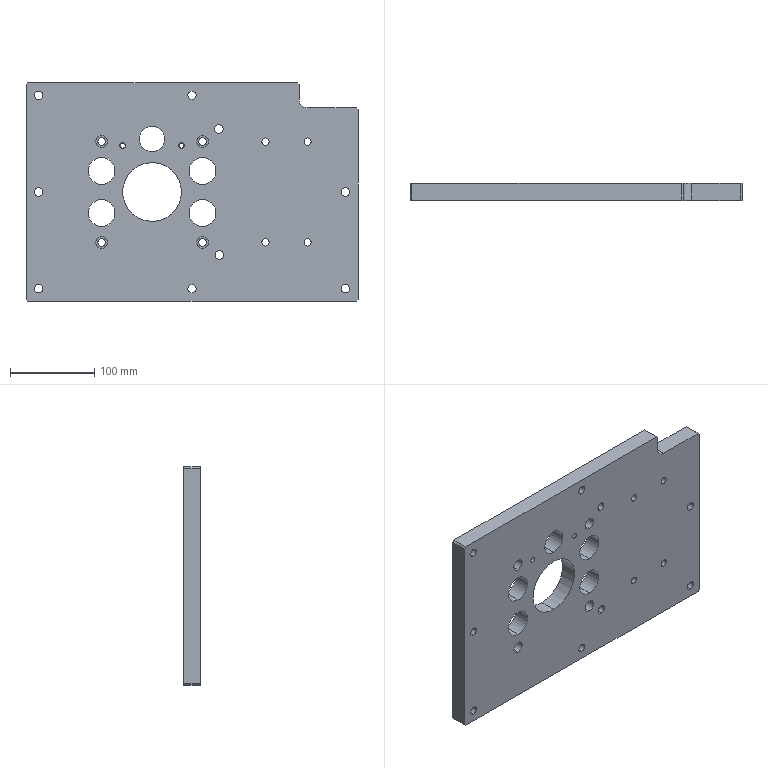Part | STEP file | (+2 more in 1 file) PN_0041 Base_Default | 1 solid | 196 faces | box 395 x 20 x 260 mm | volume 1820392 mm3 | cylinder 119 | cone 56 | plane 21 | commonest cylinder face diameters 4.2 x48 10 x22 8.5 x8 9 x8 14 x8 16 x8